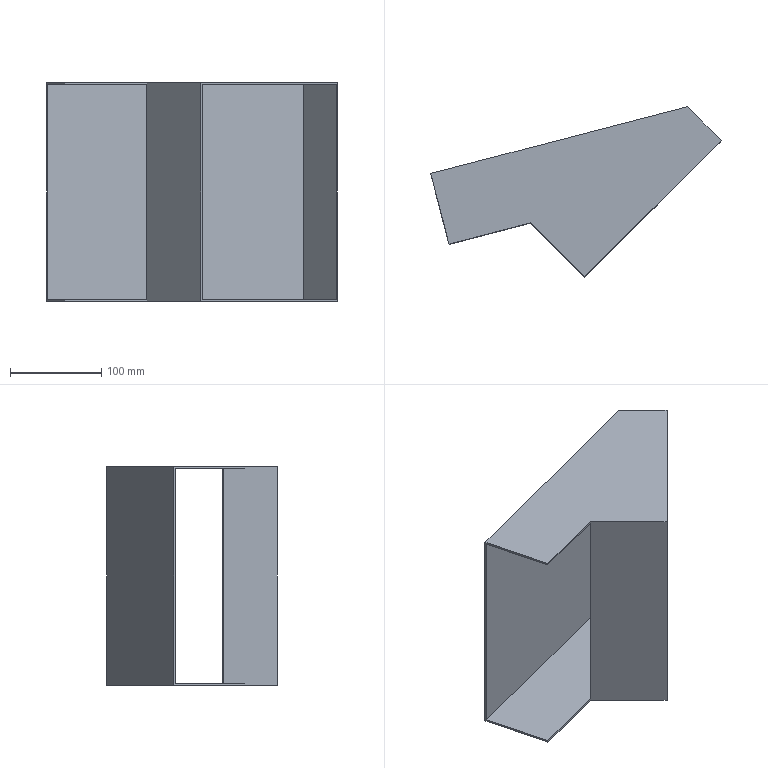Part | SolidWorks | 1 solid | 15 faces | box 318.967 x 186.877 x 240 mm | volume 339701 mm3 | plane 15
STEP:
#1=CARTESIAN_POINT('',(-383.886,160.438,-1227.42));
#2=VERTEX_POINT('',#1);
#3=CARTESIAN_POINT('',(-383.886,160.438,-991.42));
#4=VERTEX_POINT('',#3);
#5=CARTESIAN_POINT('',(-383.886,160.438,-1227.42));
#6=DIRECTION('',(0.,0.,1.));
#7=VECTOR('',#6,1000.);
#8=LINE('',#5,#7);
#9=EDGE_CURVE('',#2,#4,#8,.T.);
#10=ORIENTED_EDGE('',*,*,#9,.T.);
#11=CARTESIAN_POINT('',(-325.74,102.292,-991.42));
#12=VERTEX_POINT('',#11);
#13=CARTESIAN_POINT('',(-383.886,160.438,-991.42));
#14=DIRECTION('',(0.7071,-0.7071,0.));
#15=VECTOR('',#14,1000.);
#16=LINE('',#13,#15);
#17=EDGE_CURVE('',#4,#12,#16,.T.);
#18=ORIENTED_EDGE('',*,*,#17,.T.);
#19=CARTESIAN_POINT('',(-325.74,102.292,-1227.42));
#20=VERTEX_POINT('',#19);
#21=CARTESIAN_POINT('',(-325.74,102.292,-1227.42));
#22=DIRECTION('',(0.,0.,1.));
#23=VECTOR('',#22,1000.);
#24=LINE('',#21,#23);
#25=EDGE_CURVE('',#20,#12,#24,.T.);
#26=ORIENTED_EDGE('',*,*,#25,.F.);
#27=CARTESIAN_POINT('',(-325.74,102.292,-1227.42));
#28=DIRECTION('',(-0.7071,0.7071,0.));
#29=VECTOR('',#28,1000.);
#30=LINE('',#27,#29);
#31=EDGE_CURVE('',#20,#2,#30,.T.);
#32=ORIENTED_EDGE('',*,*,#31,.T.);
#33=EDGE_LOOP('',(#10,#18,#26,#32));
#34=FACE_OUTER_BOUND('',#33,.T.);
#35=CARTESIAN_POINT('',(-383.886,160.438,-1229.42));
#36=DIRECTION('',(0.7071,0.7071,0.));
#37=DIRECTION('',(0.7071,-0.7071,0.));
#38=AXIS2_PLACEMENT_3D('',#35,#36,#37);
#39=PLANE('',#38);
#40=ADVANCED_FACE('',(#34),#39,.T.);
#41=CARTESIAN_POINT('',(-214.867,287.048,-989.42));
#42=VERTEX_POINT('',#41);
#43=CARTESIAN_POINT('',(-177.925,250.106,-989.42));
#44=VERTEX_POINT('',#43);
#45=CARTESIAN_POINT('',(-214.867,287.048,-989.42));
#46=DIRECTION('',(0.7071,-0.7071,0.));
#47=VECTOR('',#46,1000.);
#48=LINE('',#45,#47);
#49=EDGE_CURVE('',#42,#44,#48,.T.);
#50=ORIENTED_EDGE('',*,*,#49,.T.);
#51=CARTESIAN_POINT('',(-177.925,250.106,-1229.42));
#52=VERTEX_POINT('',#51);
#53=CARTESIAN_POINT('',(-177.925,250.106,-989.42));
#54=DIRECTION('',(0.,0.,-1.));
#55=VECTOR('',#54,1000.);
#56=LINE('',#53,#55);
#57=EDGE_CURVE('',#44,#52,#56,.T.);
#58=ORIENTED_EDGE('',*,*,#57,.T.);
#59=CARTESIAN_POINT('',(-214.867,287.048,-1229.42));
#60=VERTEX_POINT('',#59);
#61=CARTESIAN_POINT('',(-177.925,250.106,-1229.42));
#62=DIRECTION('',(-0.7071,0.7071,0.));
#63=VECTOR('',#62,1000.);
#64=LINE('',#61,#63);
#65=EDGE_CURVE('',#52,#60,#64,.T.);
#66=ORIENTED_EDGE('',*,*,#65,.T.);
#67=CARTESIAN_POINT('',(-214.867,287.048,-989.42));
#68=DIRECTION('',(0.,0.,-1.));
#69=VECTOR('',#68,1000.);
#70=LINE('',#67,#69);
#71=EDGE_CURVE('',#42,#60,#70,.T.);
#72=ORIENTED_EDGE('',*,*,#71,.F.);
#73=EDGE_LOOP('',(#50,#58,#66,#72));
#74=FACE_OUTER_BOUND('',#73,.T.);
#75=CARTESIAN_POINT('',(-214.867,287.048,-1229.42));
#76=DIRECTION('',(0.7071,0.7071,0.));
#77=DIRECTION('',(0.,0.,-1.));
#78=AXIS2_PLACEMENT_3D('',#75,#76,#77);
#79=PLANE('',#78);
#80=ADVANCED_FACE('',(#74),#79,.T.);
#81=CARTESIAN_POINT('',(-476.759,136.288,-1229.42));
#82=VERTEX_POINT('',#81);
#83=CARTESIAN_POINT('',(-387.253,159.562,-1229.42));
#84=VERTEX_POINT('',#83);
#85=CARTESIAN_POINT('',(-476.759,136.288,-1229.42));
#86=DIRECTION('',(0.9678,0.2517,0.));
#87=VECTOR('',#86,1000.);
#88=LINE('',#85,#87);
#89=EDGE_CURVE('',#82,#84,#88,.T.);
#90=ORIENTED_EDGE('',*,*,#89,.T.);
#91=CARTESIAN_POINT('',(-387.253,159.562,-1227.42));
#92=VERTEX_POINT('',#91);
#93=CARTESIAN_POINT('',(-387.253,159.562,-1229.42));
#94=DIRECTION('',(0.,0.,1.));
#95=VECTOR('',#94,1000.);
#96=LINE('',#93,#95);
#97=EDGE_CURVE('',#84,#92,#96,.T.);
#98=ORIENTED_EDGE('',*,*,#97,.T.);
#99=CARTESIAN_POINT('',(-476.759,136.288,-1227.42));
#100=VERTEX_POINT('',#99);
#101=CARTESIAN_POINT('',(-387.253,159.562,-1227.42));
#102=DIRECTION('',(-0.9678,-0.2517,0.));
#103=VECTOR('',#102,1000.);
#104=LINE('',#101,#103);
#105=EDGE_CURVE('',#92,#100,#104,.T.);
#106=ORIENTED_EDGE('',*,*,#105,.T.);
#107=CARTESIAN_POINT('',(-476.759,136.288,-1227.42));
#108=DIRECTION('',(0.,0.,-1.));
#109=VECTOR('',#108,1000.);
#110=LINE('',#107,#109);
#111=EDGE_CURVE('',#100,#82,#110,.T.);
#112=ORIENTED_EDGE('',*,*,#111,.T.);
#113=EDGE_LOOP('',(#90,#98,#106,#112));
#114=FACE_OUTER_BOUND('',#113,.T.);
#115=CARTESIAN_POINT('',(-476.759,136.288,-1229.42));
#116=DIRECTION('',(0.2517,-0.9678,0.));
#117=DIRECTION('',(0.,0.,-1.));
#118=AXIS2_PLACEMENT_3D('',#115,#116,#117);
#119=PLANE('',#118);
#120=ADVANCED_FACE('',(#114),#119,.T.);
#121=CARTESIAN_POINT('',(-496.892,213.713,-1229.42));
#122=VERTEX_POINT('',#121);
#123=CARTESIAN_POINT('',(-214.867,287.048,-1229.42));
#124=DIRECTION('',(-0.9678,-0.2517,0.));
#125=VECTOR('',#124,1000.);
#126=LINE('',#123,#125);
#127=EDGE_CURVE('',#60,#122,#126,.T.);
#128=ORIENTED_EDGE('',*,*,#127,.F.);
#129=ORIENTED_EDGE('',*,*,#65,.F.);
#130=CARTESIAN_POINT('',(-327.861,100.17,-1229.42));
#131=VERTEX_POINT('',#130);
#132=CARTESIAN_POINT('',(-327.861,100.17,-1229.42));
#133=DIRECTION('',(0.7071,0.7071,0.));
#134=VECTOR('',#133,1000.);
#135=LINE('',#132,#134);
#136=EDGE_CURVE('',#131,#52,#135,.T.);
#137=ORIENTED_EDGE('',*,*,#136,.F.);
#138=CARTESIAN_POINT('',(-387.253,159.562,-1229.42));
#139=DIRECTION('',(0.7071,-0.7071,0.));
#140=VECTOR('',#139,1000.);
#141=LINE('',#138,#140);
#142=EDGE_CURVE('',#84,#131,#141,.T.);
#143=ORIENTED_EDGE('',*,*,#142,.F.);
#144=ORIENTED_EDGE('',*,*,#89,.F.);
#145=CARTESIAN_POINT('',(-496.892,213.713,-1229.42));
#146=DIRECTION('',(0.2517,-0.9678,0.));
#147=VECTOR('',#146,1000.);
#148=LINE('',#145,#147);
#149=EDGE_CURVE('',#122,#82,#148,.T.);
#150=ORIENTED_EDGE('',*,*,#149,.F.);
#151=EDGE_LOOP('',(#128,#129,#137,#143,#144,#150));
#152=FACE_OUTER_BOUND('',#151,.T.);
#153=CARTESIAN_POINT('',(0.,0.,-1229.42));
#154=DIRECTION('',(0.,0.,-1.));
#155=DIRECTION('',(0.,-1.,0.));
#156=AXIS2_PLACEMENT_3D('',#153,#154,#155);
#157=PLANE('',#156);
#158=ADVANCED_FACE('',(#152),#157,.T.);
#159=CARTESIAN_POINT('',(-496.892,213.713,-989.42));
#160=VERTEX_POINT('',#159);
#161=CARTESIAN_POINT('',(-496.892,213.713,-989.42));
#162=DIRECTION('',(0.9678,0.2517,0.));
#163=VECTOR('',#162,1000.);
#164=LINE('',#161,#163);
#165=EDGE_CURVE('',#160,#42,#164,.T.);
#166=ORIENTED_EDGE('',*,*,#165,.T.);
#167=ORIENTED_EDGE('',*,*,#71,.T.);
#168=ORIENTED_EDGE('',*,*,#127,.T.);
#169=CARTESIAN_POINT('',(-496.892,213.713,-1229.42));
#170=DIRECTION('',(0.,0.,1.));
#171=VECTOR('',#170,1000.);
#172=LINE('',#169,#171);
#173=EDGE_CURVE('',#122,#160,#172,.T.);
#174=ORIENTED_EDGE('',*,*,#173,.T.);
#175=EDGE_LOOP('',(#166,#167,#168,#174));
#176=FACE_OUTER_BOUND('',#175,.T.);
#177=CARTESIAN_POINT('',(-585.229,190.743,-1229.42));
#178=DIRECTION('',(-0.2517,0.9678,0.));
#179=DIRECTION('',(0.,0.,1.));
#180=AXIS2_PLACEMENT_3D('',#177,#178,#179);
#181=PLANE('',#180);
#182=ADVANCED_FACE('',(#176),#181,.T.);
#183=CARTESIAN_POINT('',(-387.253,159.562,-989.42));
#184=VERTEX_POINT('',#183);
#185=CARTESIAN_POINT('',(-476.759,136.288,-989.42));
#186=VERTEX_POINT('',#185);
#187=CARTESIAN_POINT('',(-387.253,159.562,-989.42));
#188=DIRECTION('',(-0.9678,-0.2517,0.));
#189=VECTOR('',#188,1000.);
#190=LINE('',#187,#189);
#191=EDGE_CURVE('',#184,#186,#190,.T.);
#192=ORIENTED_EDGE('',*,*,#191,.F.);
#193=CARTESIAN_POINT('',(-327.861,100.17,-989.42));
#194=VERTEX_POINT('',#193);
#195=CARTESIAN_POINT('',(-327.861,100.17,-989.42));
#196=DIRECTION('',(-0.7071,0.7071,0.));
#197=VECTOR('',#196,1000.);
#198=LINE('',#195,#197);
#199=EDGE_CURVE('',#194,#184,#198,.T.);
#200=ORIENTED_EDGE('',*,*,#199,.F.);
#201=CARTESIAN_POINT('',(-177.925,250.106,-989.42));
#202=DIRECTION('',(-0.7071,-0.7071,0.));
#203=VECTOR('',#202,1000.);
#204=LINE('',#201,#203);
#205=EDGE_CURVE('',#44,#194,#204,.T.);
#206=ORIENTED_EDGE('',*,*,#205,.F.);
#207=ORIENTED_EDGE('',*,*,#49,.F.);
#208=ORIENTED_EDGE('',*,*,#165,.F.);
#209=CARTESIAN_POINT('',(-476.759,136.288,-989.42));
#210=DIRECTION('',(-0.2517,0.9678,0.));
#211=VECTOR('',#210,1000.);
#212=LINE('',#209,#211);
#213=EDGE_CURVE('',#186,#160,#212,.T.);
#214=ORIENTED_EDGE('',*,*,#213,.F.);
#215=EDGE_LOOP('',(#192,#200,#206,#207,#208,#214));
#216=FACE_OUTER_BOUND('',#215,.T.);
#217=CARTESIAN_POINT('',(63.64,134.35,-989.42));
#218=DIRECTION('',(0.,0.,1.));
#219=DIRECTION('',(1.,0.,0.));
#220=AXIS2_PLACEMENT_3D('',#217,#218,#219);
#221=PLANE('',#220);
#222=ADVANCED_FACE('',(#216),#221,.T.);
#223=ORIENTED_EDGE('',*,*,#97,.F.);
#224=ORIENTED_EDGE('',*,*,#142,.T.);
#225=CARTESIAN_POINT('',(-327.861,100.17,-989.42));
#226=DIRECTION('',(0.,0.,-1.));
#227=VECTOR('',#226,1000.);
#228=LINE('',#225,#227);
#229=EDGE_CURVE('',#194,#131,#228,.T.);
#230=ORIENTED_EDGE('',*,*,#229,.F.);
#231=ORIENTED_EDGE('',*,*,#199,.T.);
#232=CARTESIAN_POINT('',(-387.253,159.562,-991.42));
#233=VERTEX_POINT('',#232);
#234=CARTESIAN_POINT('',(-387.253,159.562,-991.42));
#235=DIRECTION('',(0.,0.,1.));
#236=VECTOR('',#235,1000.);
#237=LINE('',#234,#236);
#238=EDGE_CURVE('',#233,#184,#237,.T.);
#239=ORIENTED_EDGE('',*,*,#238,.F.);
#240=CARTESIAN_POINT('',(-387.253,159.562,-1227.42));
#241=DIRECTION('',(0.,0.,1.));
#242=VECTOR('',#241,1000.);
#243=LINE('',#240,#242);
#244=EDGE_CURVE('',#92,#233,#243,.T.);
#245=ORIENTED_EDGE('',*,*,#244,.F.);
#246=EDGE_LOOP('',(#223,#224,#230,#231,#239,#245));
#247=FACE_OUTER_BOUND('',#246,.T.);
#248=CARTESIAN_POINT('',(-327.861,100.17,-1229.42));
#249=DIRECTION('',(-0.7071,-0.7071,0.));
#250=DIRECTION('',(-0.7071,0.7071,0.));
#251=AXIS2_PLACEMENT_3D('',#248,#249,#250);
#252=PLANE('',#251);
#253=ADVANCED_FACE('',(#247),#252,.T.);
#254=CARTESIAN_POINT('',(-179.34,248.692,-1227.42));
#255=VERTEX_POINT('',#254);
#256=CARTESIAN_POINT('',(-179.34,248.692,-991.42));
#257=VERTEX_POINT('',#256);
#258=CARTESIAN_POINT('',(-179.34,248.692,-1227.42));
#259=DIRECTION('',(0.,0.,1.));
#260=VECTOR('',#259,1000.);
#261=LINE('',#258,#260);
#262=EDGE_CURVE('',#255,#257,#261,.T.);
#263=ORIENTED_EDGE('',*,*,#262,.F.);
#264=CARTESIAN_POINT('',(-179.34,248.692,-1227.42));
#265=DIRECTION('',(-0.7071,-0.7071,0.));
#266=VECTOR('',#265,1000.);
#267=LINE('',#264,#266);
#268=EDGE_CURVE('',#255,#20,#267,.T.);
#269=ORIENTED_EDGE('',*,*,#268,.T.);
#270=ORIENTED_EDGE('',*,*,#25,.T.);
#271=CARTESIAN_POINT('',(-325.74,102.292,-991.42));
#272=DIRECTION('',(0.7071,0.7071,0.));
#273=VECTOR('',#272,1000.);
#274=LINE('',#271,#273);
#275=EDGE_CURVE('',#12,#257,#274,.T.);
#276=ORIENTED_EDGE('',*,*,#275,.T.);
#277=EDGE_LOOP('',(#263,#269,#270,#276));
#278=FACE_BOUND('',#277,.T.);
#279=ORIENTED_EDGE('',*,*,#136,.T.);
#280=ORIENTED_EDGE('',*,*,#57,.F.);
#281=ORIENTED_EDGE('',*,*,#205,.T.);
#282=ORIENTED_EDGE('',*,*,#229,.T.);
#283=EDGE_LOOP('',(#279,#280,#281,#282));
#284=FACE_OUTER_BOUND('',#283,.T.);
#285=CARTESIAN_POINT('',(-177.925,250.106,-1229.42));
#286=DIRECTION('',(0.7071,-0.7071,0.));
#287=DIRECTION('',(0.,0.,-1.));
#288=AXIS2_PLACEMENT_3D('',#285,#286,#287);
#289=PLANE('',#288);
#290=ADVANCED_FACE('',(#278,#284),#289,.T.);
#291=CARTESIAN_POINT('',(-215.472,284.824,-991.42));
#292=VERTEX_POINT('',#291);
#293=CARTESIAN_POINT('',(-215.472,284.824,-1227.42));
#294=VERTEX_POINT('',#293);
#295=CARTESIAN_POINT('',(-215.472,284.824,-991.42));
#296=DIRECTION('',(0.,0.,-1.));
#297=VECTOR('',#296,1000.);
#298=LINE('',#295,#297);
#299=EDGE_CURVE('',#292,#294,#298,.T.);
#300=ORIENTED_EDGE('',*,*,#299,.T.);
#301=CARTESIAN_POINT('',(-215.472,284.824,-1227.42));
#302=DIRECTION('',(0.7071,-0.7071,0.));
#303=VECTOR('',#302,1000.);
#304=LINE('',#301,#303);
#305=EDGE_CURVE('',#294,#255,#304,.T.);
#306=ORIENTED_EDGE('',*,*,#305,.T.);
#307=ORIENTED_EDGE('',*,*,#262,.T.);
#308=CARTESIAN_POINT('',(-179.34,248.692,-991.42));
#309=DIRECTION('',(-0.7071,0.7071,0.));
#310=VECTOR('',#309,1000.);
#311=LINE('',#308,#310);
#312=EDGE_CURVE('',#257,#292,#311,.T.);
#313=ORIENTED_EDGE('',*,*,#312,.T.);
#314=EDGE_LOOP('',(#300,#306,#307,#313));
#315=FACE_OUTER_BOUND('',#314,.T.);
#316=CARTESIAN_POINT('',(-216.281,285.633,-1229.42));
#317=DIRECTION('',(0.7071,0.7071,0.));
#318=DIRECTION('',(0.,0.,-1.));
#319=AXIS2_PLACEMENT_3D('',#316,#317,#318);
#320=PLANE('',#319);
#321=ADVANCED_FACE('',(#315),#320,.F.);
#322=CARTESIAN_POINT('',(-496.389,211.777,-1227.42));
#323=VERTEX_POINT('',#322);
#324=CARTESIAN_POINT('',(-496.389,211.777,-1227.42));
#325=DIRECTION('',(0.9678,0.2517,0.));
#326=VECTOR('',#325,1000.);
#327=LINE('',#324,#326);
#328=EDGE_CURVE('',#323,#294,#327,.T.);
#329=ORIENTED_EDGE('',*,*,#328,.T.);
#330=ORIENTED_EDGE('',*,*,#299,.F.);
#331=CARTESIAN_POINT('',(-496.389,211.777,-991.42));
#332=VERTEX_POINT('',#331);
#333=CARTESIAN_POINT('',(-215.472,284.824,-991.42));
#334=DIRECTION('',(-0.9678,-0.2517,0.));
#335=VECTOR('',#334,1000.);
#336=LINE('',#333,#335);
#337=EDGE_CURVE('',#292,#332,#336,.T.);
#338=ORIENTED_EDGE('',*,*,#337,.T.);
#339=CARTESIAN_POINT('',(-496.389,211.777,-1227.42));
#340=DIRECTION('',(0.,0.,1.));
#341=VECTOR('',#340,1000.);
#342=LINE('',#339,#341);
#343=EDGE_CURVE('',#323,#332,#342,.T.);
#344=ORIENTED_EDGE('',*,*,#343,.F.);
#345=EDGE_LOOP('',(#329,#330,#338,#344));
#346=FACE_OUTER_BOUND('',#345,.T.);
#347=CARTESIAN_POINT('',(-584.725,188.807,-1229.42));
#348=DIRECTION('',(-0.2517,0.9678,0.));
#349=DIRECTION('',(0.,0.,1.));
#350=AXIS2_PLACEMENT_3D('',#347,#348,#349);
#351=PLANE('',#350);
#352=ADVANCED_FACE('',(#346),#351,.F.);
#353=ORIENTED_EDGE('',*,*,#105,.F.);
#354=CARTESIAN_POINT('',(-383.886,160.438,-1227.42));
#355=DIRECTION('',(-0.9678,-0.2517,0.));
#356=VECTOR('',#355,1000.);
#357=LINE('',#354,#356);
#358=EDGE_CURVE('',#2,#92,#357,.T.);
#359=ORIENTED_EDGE('',*,*,#358,.F.);
#360=ORIENTED_EDGE('',*,*,#31,.F.);
#361=ORIENTED_EDGE('',*,*,#268,.F.);
#362=ORIENTED_EDGE('',*,*,#305,.F.);
#363=ORIENTED_EDGE('',*,*,#328,.F.);
#364=CARTESIAN_POINT('',(-476.759,136.288,-1227.42));
#365=DIRECTION('',(-0.2517,0.9678,0.));
#366=VECTOR('',#365,1000.);
#367=LINE('',#364,#366);
#368=EDGE_CURVE('',#100,#323,#367,.T.);
#369=ORIENTED_EDGE('',*,*,#368,.F.);
#370=EDGE_LOOP('',(#353,#359,#360,#361,#362,#363,#369));
#371=FACE_OUTER_BOUND('',#370,.T.);
#372=CARTESIAN_POINT('',(0.,0.,-1227.42));
#373=DIRECTION('',(0.,0.,-1.));
#374=DIRECTION('',(0.,-1.,0.));
#375=AXIS2_PLACEMENT_3D('',#372,#373,#374);
#376=PLANE('',#375);
#377=ADVANCED_FACE('',(#371),#376,.F.);
#378=ORIENTED_EDGE('',*,*,#244,.T.);
#379=CARTESIAN_POINT('',(-387.253,159.562,-991.42));
#380=DIRECTION('',(0.9678,0.2517,0.));
#381=VECTOR('',#380,1000.);
#382=LINE('',#379,#381);
#383=EDGE_CURVE('',#233,#4,#382,.T.);
#384=ORIENTED_EDGE('',*,*,#383,.T.);
#385=ORIENTED_EDGE('',*,*,#9,.F.);
#386=ORIENTED_EDGE('',*,*,#358,.T.);
#387=EDGE_LOOP('',(#378,#384,#385,#386));
#388=FACE_OUTER_BOUND('',#387,.T.);
#389=CARTESIAN_POINT('',(-387.253,159.562,-1229.42));
#390=DIRECTION('',(-0.2517,0.9678,0.));
#391=DIRECTION('',(0.9678,0.2517,0.));
#392=AXIS2_PLACEMENT_3D('',#389,#390,#391);
#393=PLANE('',#392);
#394=ADVANCED_FACE('',(#388),#393,.T.);
#395=ORIENTED_EDGE('',*,*,#337,.F.);
#396=ORIENTED_EDGE('',*,*,#312,.F.);
#397=ORIENTED_EDGE('',*,*,#275,.F.);
#398=ORIENTED_EDGE('',*,*,#17,.F.);
#399=ORIENTED_EDGE('',*,*,#383,.F.);
#400=CARTESIAN_POINT('',(-476.759,136.288,-991.42));
#401=VERTEX_POINT('',#400);
#402=CARTESIAN_POINT('',(-476.759,136.288,-991.42));
#403=DIRECTION('',(0.9678,0.2517,0.));
#404=VECTOR('',#403,1000.);
#405=LINE('',#402,#404);
#406=EDGE_CURVE('',#401,#233,#405,.T.);
#407=ORIENTED_EDGE('',*,*,#406,.F.);
#408=CARTESIAN_POINT('',(-496.389,211.777,-991.42));
#409=DIRECTION('',(0.2517,-0.9678,0.));
#410=VECTOR('',#409,1000.);
#411=LINE('',#408,#410);
#412=EDGE_CURVE('',#332,#401,#411,.T.);
#413=ORIENTED_EDGE('',*,*,#412,.F.);
#414=EDGE_LOOP('',(#395,#396,#397,#398,#399,#407,#413));
#415=FACE_OUTER_BOUND('',#414,.T.);
#416=CARTESIAN_POINT('',(63.64,134.35,-991.42));
#417=DIRECTION('',(0.,0.,1.));
#418=DIRECTION('',(1.,0.,0.));
#419=AXIS2_PLACEMENT_3D('',#416,#417,#418);
#420=PLANE('',#419);
#421=ADVANCED_FACE('',(#415),#420,.F.);
#422=ORIENTED_EDGE('',*,*,#213,.T.);
#423=ORIENTED_EDGE('',*,*,#173,.F.);
#424=ORIENTED_EDGE('',*,*,#149,.T.);
#425=ORIENTED_EDGE('',*,*,#111,.F.);
#426=ORIENTED_EDGE('',*,*,#368,.T.);
#427=ORIENTED_EDGE('',*,*,#343,.T.);
#428=ORIENTED_EDGE('',*,*,#412,.T.);
#429=CARTESIAN_POINT('',(-476.759,136.288,-989.42));
#430=DIRECTION('',(0.,0.,-1.));
#431=VECTOR('',#430,1000.);
#432=LINE('',#429,#431);
#433=EDGE_CURVE('',#186,#401,#432,.T.);
#434=ORIENTED_EDGE('',*,*,#433,.F.);
#435=EDGE_LOOP('',(#422,#423,#424,#425,#426,#427,#428,#434));
#436=FACE_OUTER_BOUND('',#435,.T.);
#437=CARTESIAN_POINT('',(-476.759,136.288,-989.42));
#438=DIRECTION('',(0.9678,0.2517,0.));
#439=DIRECTION('',(-0.2517,0.9678,0.));
#440=AXIS2_PLACEMENT_3D('',#437,#438,#439);
#441=PLANE('',#440);
#442=ADVANCED_FACE('',(#436),#441,.F.);
#443=ORIENTED_EDGE('',*,*,#406,.T.);
#444=ORIENTED_EDGE('',*,*,#238,.T.);
#445=ORIENTED_EDGE('',*,*,#191,.T.);
#446=ORIENTED_EDGE('',*,*,#433,.T.);
#447=EDGE_LOOP('',(#443,#444,#445,#446));
#448=FACE_OUTER_BOUND('',#447,.T.);
#449=CARTESIAN_POINT('',(-476.759,136.288,-1229.42));
#450=DIRECTION('',(0.2517,-0.9678,0.));
#451=DIRECTION('',(0.,0.,-1.));
#452=AXIS2_PLACEMENT_3D('',#449,#450,#451);
#453=PLANE('',#452);
#454=ADVANCED_FACE('',(#448),#453,.T.);
#455=CLOSED_SHELL('',(#40,#80,#120,#158,#182,#222,#253,#290,#321,#352,#377,#394,#421,#442,#454));
#456=MANIFOLD_SOLID_BREP('',#455);
#457=CARTESIAN_POINT('',(0.,0.,0.));
#458=DIRECTION('',(0.,0.,1.));
#459=DIRECTION('',(1.,0.,0.));
#460=AXIS2_PLACEMENT_3D('',#457,#458,#459);
#461=(LENGTH_UNIT()NAMED_UNIT(*)SI_UNIT(.MILLI.,.METRE.));
#462=UNCERTAINTY_MEASURE_WITH_UNIT(LENGTH_MEASURE(0.00001),#461,'','');
#463=(NAMED_UNIT(*)PLANE_ANGLE_UNIT()SI_UNIT($,.RADIAN.));
#464=(NAMED_UNIT(*)SI_UNIT($,.STERADIAN.)SOLID_ANGLE_UNIT());
#465=(GEOMETRIC_REPRESENTATION_CONTEXT(3)GLOBAL_UNCERTAINTY_ASSIGNED_CONTEXT((#462))GLOBAL_UNIT_ASSIGNED_CONTEXT((#461,#463,#464))REPRESENTATION_CONTEXT('',''));
#466=ADVANCED_BREP_SHAPE_REPRESENTATION('',(#456,#460),#465);